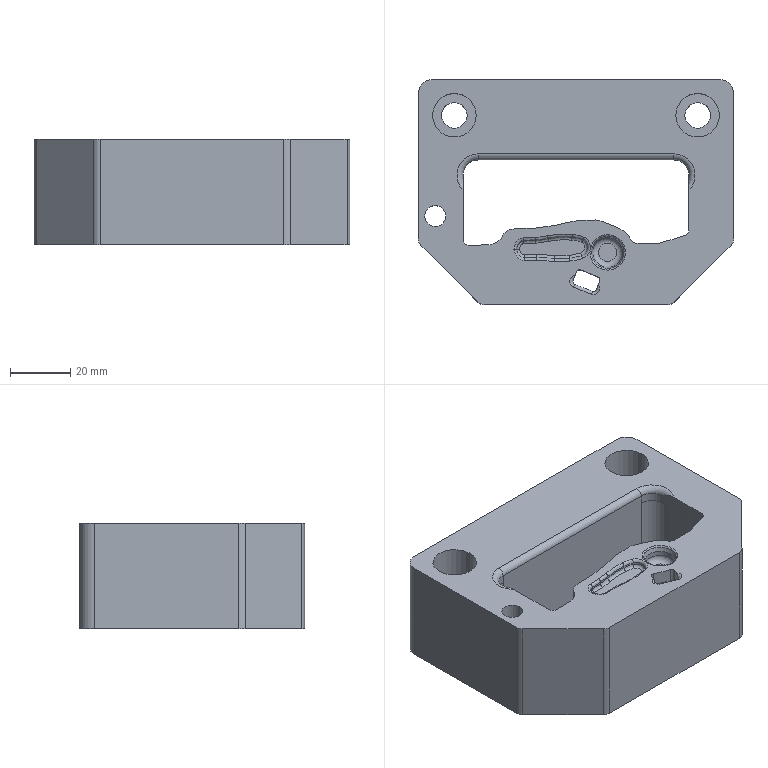Part | NX | features DIE-40 2 | 1 solid | 114 faces | box 105 x 75 x 35 mm | volume 182613 mm3 | spline 44 | cylinder 31 | plane 30 | torus 8 | sphere 1 | commonest cylinder face diameters 6 x5 4.24 x4 6.24 x4 2 x3 10 x3 2.4 x2